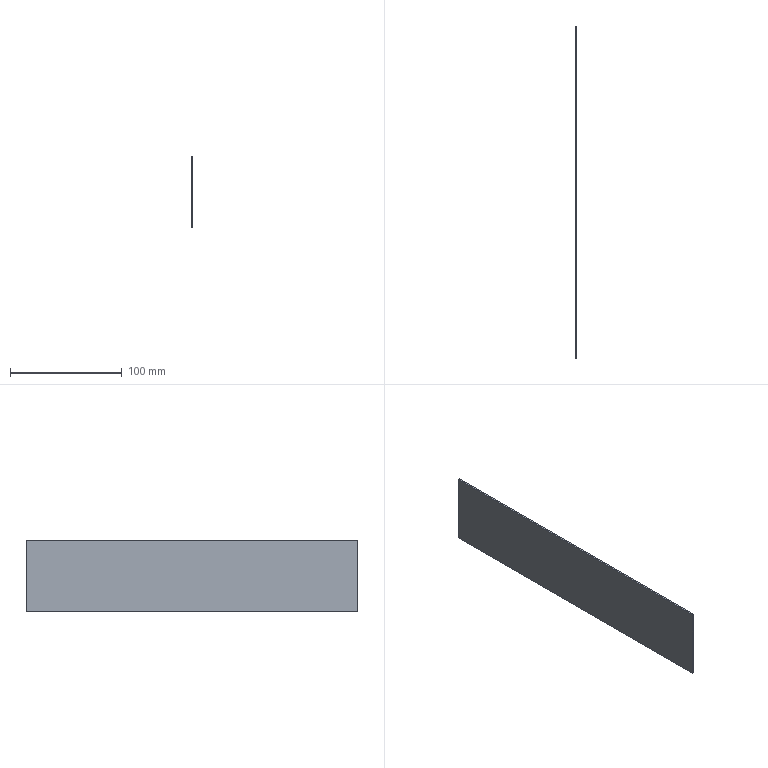Part | SolidWorks | features Extrusion 1 | 1 solid | 6 faces | box 1.5 x 297 x 64 mm | volume 28512 mm3 | plane 6
STEP:
#1=CARTESIAN_POINT('',(-0.75,148.5,-32.));
#2=VERTEX_POINT('',#1);
#3=CARTESIAN_POINT('',(-0.75,-148.5,-32.));
#4=VERTEX_POINT('',#3);
#5=CARTESIAN_POINT('',(-0.75,148.5,-32.));
#6=DIRECTION('',(0.,-1.,0.));
#7=VECTOR('',#6,1000.);
#8=LINE('',#5,#7);
#9=EDGE_CURVE('',#2,#4,#8,.T.);
#10=ORIENTED_EDGE('',*,*,#9,.T.);
#11=CARTESIAN_POINT('',(-0.75,-148.5,32.));
#12=VERTEX_POINT('',#11);
#13=CARTESIAN_POINT('',(-0.75,-148.5,32.));
#14=DIRECTION('',(0.,0.,-1.));
#15=VECTOR('',#14,1000.);
#16=LINE('',#13,#15);
#17=EDGE_CURVE('',#12,#4,#16,.T.);
#18=ORIENTED_EDGE('',*,*,#17,.F.);
#19=CARTESIAN_POINT('',(-0.75,148.5,32.));
#20=VERTEX_POINT('',#19);
#21=CARTESIAN_POINT('',(-0.75,148.5,32.));
#22=DIRECTION('',(0.,-1.,0.));
#23=VECTOR('',#22,1000.);
#24=LINE('',#21,#23);
#25=EDGE_CURVE('',#20,#12,#24,.T.);
#26=ORIENTED_EDGE('',*,*,#25,.F.);
#27=CARTESIAN_POINT('',(-0.75,148.5,32.));
#28=DIRECTION('',(0.,0.,-1.));
#29=VECTOR('',#28,1000.);
#30=LINE('',#27,#29);
#31=EDGE_CURVE('',#20,#2,#30,.T.);
#32=ORIENTED_EDGE('',*,*,#31,.T.);
#33=EDGE_LOOP('',(#10,#18,#26,#32));
#34=FACE_OUTER_BOUND('',#33,.T.);
#35=CARTESIAN_POINT('',(-0.75,148.5,32.));
#36=DIRECTION('',(1.,0.,0.));
#37=DIRECTION('',(0.,1.,0.));
#38=AXIS2_PLACEMENT_3D('',#35,#36,#37);
#39=PLANE('',#38);
#40=ADVANCED_FACE('',(#34),#39,.F.);
#41=CARTESIAN_POINT('',(0.75,-148.5,-32.));
#42=VERTEX_POINT('',#41);
#43=CARTESIAN_POINT('',(0.75,-148.5,-32.));
#44=DIRECTION('',(1.,0.,0.));
#45=VECTOR('',#44,1000.);
#46=LINE('',#43,#45);
#47=EDGE_CURVE('',#4,#42,#46,.T.);
#48=ORIENTED_EDGE('',*,*,#47,.T.);
#49=CARTESIAN_POINT('',(0.75,-148.5,32.));
#50=VERTEX_POINT('',#49);
#51=CARTESIAN_POINT('',(0.75,-148.5,32.));
#52=DIRECTION('',(0.,0.,-1.));
#53=VECTOR('',#52,1000.);
#54=LINE('',#51,#53);
#55=EDGE_CURVE('',#50,#42,#54,.T.);
#56=ORIENTED_EDGE('',*,*,#55,.F.);
#57=CARTESIAN_POINT('',(0.75,-148.5,32.));
#58=DIRECTION('',(1.,0.,0.));
#59=VECTOR('',#58,1000.);
#60=LINE('',#57,#59);
#61=EDGE_CURVE('',#12,#50,#60,.T.);
#62=ORIENTED_EDGE('',*,*,#61,.F.);
#63=ORIENTED_EDGE('',*,*,#17,.T.);
#64=EDGE_LOOP('',(#48,#56,#62,#63));
#65=FACE_OUTER_BOUND('',#64,.T.);
#66=CARTESIAN_POINT('',(0.75,-148.5,32.));
#67=DIRECTION('',(0.,1.,0.));
#68=DIRECTION('',(0.,0.,1.));
#69=AXIS2_PLACEMENT_3D('',#66,#67,#68);
#70=PLANE('',#69);
#71=ADVANCED_FACE('',(#65),#70,.F.);
#72=CARTESIAN_POINT('',(0.75,148.5,-32.));
#73=VERTEX_POINT('',#72);
#74=CARTESIAN_POINT('',(0.75,148.5,-32.));
#75=DIRECTION('',(0.,1.,0.));
#76=VECTOR('',#75,1000.);
#77=LINE('',#74,#76);
#78=EDGE_CURVE('',#42,#73,#77,.T.);
#79=ORIENTED_EDGE('',*,*,#78,.T.);
#80=CARTESIAN_POINT('',(0.75,148.5,32.));
#81=VERTEX_POINT('',#80);
#82=CARTESIAN_POINT('',(0.75,148.5,32.));
#83=DIRECTION('',(0.,0.,-1.));
#84=VECTOR('',#83,1000.);
#85=LINE('',#82,#84);
#86=EDGE_CURVE('',#81,#73,#85,.T.);
#87=ORIENTED_EDGE('',*,*,#86,.F.);
#88=CARTESIAN_POINT('',(0.75,148.5,32.));
#89=DIRECTION('',(0.,1.,0.));
#90=VECTOR('',#89,1000.);
#91=LINE('',#88,#90);
#92=EDGE_CURVE('',#50,#81,#91,.T.);
#93=ORIENTED_EDGE('',*,*,#92,.F.);
#94=ORIENTED_EDGE('',*,*,#55,.T.);
#95=EDGE_LOOP('',(#79,#87,#93,#94));
#96=FACE_OUTER_BOUND('',#95,.T.);
#97=CARTESIAN_POINT('',(0.75,148.5,32.));
#98=DIRECTION('',(-1.,0.,0.));
#99=DIRECTION('',(0.,-1.,0.));
#100=AXIS2_PLACEMENT_3D('',#97,#98,#99);
#101=PLANE('',#100);
#102=ADVANCED_FACE('',(#96),#101,.F.);
#103=CARTESIAN_POINT('',(0.75,148.5,-32.));
#104=DIRECTION('',(-1.,0.,0.));
#105=VECTOR('',#104,1000.);
#106=LINE('',#103,#105);
#107=EDGE_CURVE('',#73,#2,#106,.T.);
#108=ORIENTED_EDGE('',*,*,#107,.T.);
#109=ORIENTED_EDGE('',*,*,#31,.F.);
#110=CARTESIAN_POINT('',(0.75,148.5,32.));
#111=DIRECTION('',(-1.,0.,0.));
#112=VECTOR('',#111,1000.);
#113=LINE('',#110,#112);
#114=EDGE_CURVE('',#81,#20,#113,.T.);
#115=ORIENTED_EDGE('',*,*,#114,.F.);
#116=ORIENTED_EDGE('',*,*,#86,.T.);
#117=EDGE_LOOP('',(#108,#109,#115,#116));
#118=FACE_OUTER_BOUND('',#117,.T.);
#119=CARTESIAN_POINT('',(0.75,148.5,32.));
#120=DIRECTION('',(0.,-1.,0.));
#121=DIRECTION('',(0.,0.,-1.));
#122=AXIS2_PLACEMENT_3D('',#119,#120,#121);
#123=PLANE('',#122);
#124=ADVANCED_FACE('',(#118),#123,.F.);
#125=ORIENTED_EDGE('',*,*,#25,.T.);
#126=ORIENTED_EDGE('',*,*,#61,.T.);
#127=ORIENTED_EDGE('',*,*,#92,.T.);
#128=ORIENTED_EDGE('',*,*,#114,.T.);
#129=EDGE_LOOP('',(#125,#126,#127,#128));
#130=FACE_OUTER_BOUND('',#129,.T.);
#131=CARTESIAN_POINT('',(0.,0.,32.));
#132=DIRECTION('',(0.,0.,-1.));
#133=DIRECTION('',(-1.,0.,0.));
#134=AXIS2_PLACEMENT_3D('',#131,#132,#133);
#135=PLANE('',#134);
#136=ADVANCED_FACE('',(#130),#135,.F.);
#137=ORIENTED_EDGE('',*,*,#9,.F.);
#138=ORIENTED_EDGE('',*,*,#107,.F.);
#139=ORIENTED_EDGE('',*,*,#78,.F.);
#140=ORIENTED_EDGE('',*,*,#47,.F.);
#141=EDGE_LOOP('',(#137,#138,#139,#140));
#142=FACE_OUTER_BOUND('',#141,.T.);
#143=CARTESIAN_POINT('',(0.,0.,-32.));
#144=DIRECTION('',(0.,0.,-1.));
#145=DIRECTION('',(-1.,0.,0.));
#146=AXIS2_PLACEMENT_3D('',#143,#144,#145);
#147=PLANE('',#146);
#148=ADVANCED_FACE('',(#142),#147,.T.);
#149=CLOSED_SHELL('',(#40,#71,#102,#124,#136,#148));
#150=MANIFOLD_SOLID_BREP('',#149);
#151=CARTESIAN_POINT('',(0.,0.,0.));
#152=DIRECTION('',(0.,0.,1.));
#153=DIRECTION('',(1.,0.,0.));
#154=AXIS2_PLACEMENT_3D('',#151,#152,#153);
#155=(LENGTH_UNIT()NAMED_UNIT(*)SI_UNIT(.MILLI.,.METRE.));
#156=UNCERTAINTY_MEASURE_WITH_UNIT(LENGTH_MEASURE(0.00001),#155,'','');
#157=(NAMED_UNIT(*)PLANE_ANGLE_UNIT()SI_UNIT($,.RADIAN.));
#158=(NAMED_UNIT(*)SI_UNIT($,.STERADIAN.)SOLID_ANGLE_UNIT());
#159=(GEOMETRIC_REPRESENTATION_CONTEXT(3)GLOBAL_UNCERTAINTY_ASSIGNED_CONTEXT((#156))GLOBAL_UNIT_ASSIGNED_CONTEXT((#155,#157,#158))REPRESENTATION_CONTEXT('',''));
#160=ADVANCED_BREP_SHAPE_REPRESENTATION('',(#150,#154),#159);